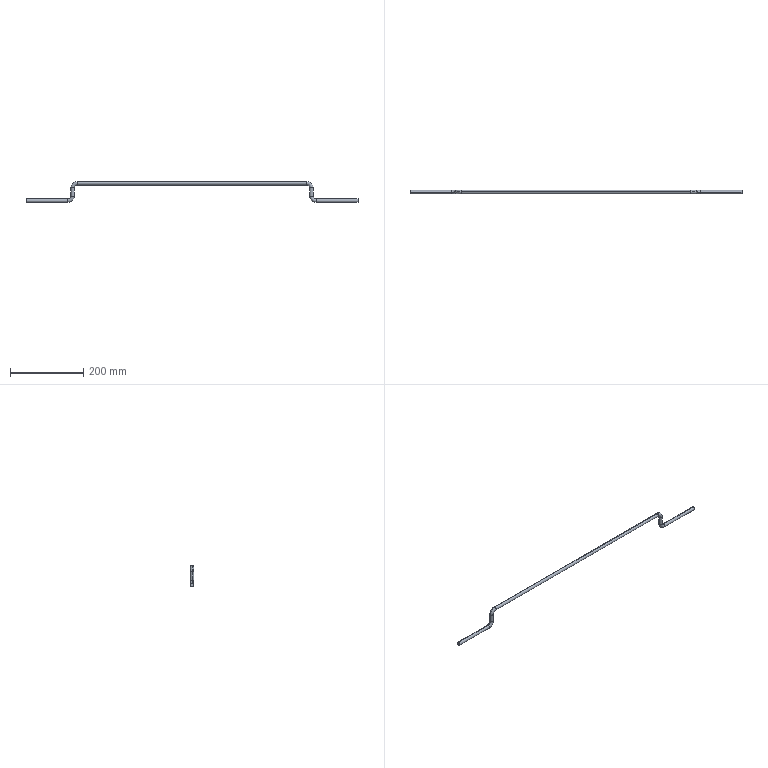Part | NX | features BREP 1 | 1 solid | 20 faces | box 904.875 x 9.525 x 57.15 mm | volume 69711 mm3 | cylinder 10 | torus 8 | plane 2 | commonest cylinder face diameters 9.525 x10
STEP:
#1=CARTESIAN_POINT('',(-452.438,0.,4.763));
#2=VERTEX_POINT('',#1);
#3=CARTESIAN_POINT('',(-452.438,0.,-4.763));
#4=VERTEX_POINT('',#3);
#5=CARTESIAN_POINT('',(-452.438,0.,0.));
#6=DIRECTION('',(1.,0.,0.));
#7=DIRECTION('',(0.,0.,1.));
#8=AXIS2_PLACEMENT_3D('',#5,#6,#7);
#9=CIRCLE('',#8,4.763);
#10=EDGE_CURVE('',#2,#4,#9,.T.);
#11=ORIENTED_EDGE('',*,*,#10,.F.);
#12=CARTESIAN_POINT('',(-452.438,0.,0.));
#13=DIRECTION('',(1.,0.,0.));
#14=DIRECTION('',(0.,0.,-1.));
#15=AXIS2_PLACEMENT_3D('',#12,#13,#14);
#16=CIRCLE('',#15,4.763);
#17=EDGE_CURVE('',#4,#2,#16,.T.);
#18=ORIENTED_EDGE('',*,*,#17,.F.);
#19=EDGE_LOOP('',(#11,#18));
#20=FACE_BOUND('',#19,.T.);
#21=CARTESIAN_POINT('',(-452.438,0.,0.));
#22=DIRECTION('',(1.,0.,0.));
#23=DIRECTION('',(0.,1.,0.));
#24=AXIS2_PLACEMENT_3D('',#21,#22,#23);
#25=PLANE('',#24);
#26=ADVANCED_FACE('',(#20),#25,.F.);
#27=CARTESIAN_POINT('',(-338.137,0.,4.763));
#28=VERTEX_POINT('',#27);
#29=CARTESIAN_POINT('',(-452.438,0.,4.763));
#30=DIRECTION('',(1.,0.,0.));
#31=VECTOR('',#30,1000.);
#32=LINE('',#29,#31);
#33=EDGE_CURVE('',#28,#2,#32,.F.);
#34=ORIENTED_EDGE('',*,*,#33,.F.);
#35=CARTESIAN_POINT('',(-338.137,0.,-4.763));
#36=VERTEX_POINT('',#35);
#37=CARTESIAN_POINT('',(-338.137,0.,0.));
#38=DIRECTION('',(1.,0.,0.));
#39=DIRECTION('',(0.,0.,-1.));
#40=AXIS2_PLACEMENT_3D('',#37,#38,#39);
#41=CIRCLE('',#40,4.763);
#42=EDGE_CURVE('',#36,#28,#41,.T.);
#43=ORIENTED_EDGE('',*,*,#42,.F.);
#44=CARTESIAN_POINT('',(-452.438,0.,-4.763));
#45=DIRECTION('',(1.,0.,0.));
#46=VECTOR('',#45,1000.);
#47=LINE('',#44,#46);
#48=EDGE_CURVE('',#36,#4,#47,.F.);
#49=ORIENTED_EDGE('',*,*,#48,.T.);
#50=ORIENTED_EDGE('',*,*,#17,.T.);
#51=EDGE_LOOP('',(#34,#43,#49,#50));
#52=FACE_BOUND('',#51,.T.);
#53=CARTESIAN_POINT('',(-452.438,0.,0.));
#54=DIRECTION('',(1.,0.,0.));
#55=DIRECTION('',(0.,0.,-1.));
#56=AXIS2_PLACEMENT_3D('',#53,#54,#55);
#57=CYLINDRICAL_SURFACE('',#56,4.763);
#58=ADVANCED_FACE('',(#52),#57,.T.);
#59=ORIENTED_EDGE('',*,*,#48,.F.);
#60=CARTESIAN_POINT('',(-338.137,0.,0.));
#61=DIRECTION('',(1.,0.,0.));
#62=DIRECTION('',(0.,0.,1.));
#63=AXIS2_PLACEMENT_3D('',#60,#61,#62);
#64=CIRCLE('',#63,4.763);
#65=EDGE_CURVE('',#28,#36,#64,.T.);
#66=ORIENTED_EDGE('',*,*,#65,.F.);
#67=ORIENTED_EDGE('',*,*,#33,.T.);
#68=ORIENTED_EDGE('',*,*,#10,.T.);
#69=EDGE_LOOP('',(#59,#66,#67,#68));
#70=FACE_BOUND('',#69,.T.);
#71=CARTESIAN_POINT('',(-452.438,0.,0.));
#72=DIRECTION('',(1.,0.,0.));
#73=DIRECTION('',(0.,0.,-1.));
#74=AXIS2_PLACEMENT_3D('',#71,#72,#73);
#75=CYLINDRICAL_SURFACE('',#74,4.763);
#76=ADVANCED_FACE('',(#70),#75,.T.);
#77=CARTESIAN_POINT('',(-320.675,0.,12.7));
#78=VERTEX_POINT('',#77);
#79=CARTESIAN_POINT('',(-338.137,0.,12.7));
#80=DIRECTION('',(0.,-1.,0.));
#81=DIRECTION('',(0.,0.,-1.));
#82=AXIS2_PLACEMENT_3D('',#79,#80,#81);
#83=CIRCLE('',#82,17.462);
#84=EDGE_CURVE('',#36,#78,#83,.T.);
#85=ORIENTED_EDGE('',*,*,#84,.T.);
#86=CARTESIAN_POINT('',(-330.2,0.,12.7));
#87=VERTEX_POINT('',#86);
#88=CARTESIAN_POINT('',(-325.438,0.,12.7));
#89=DIRECTION('',(0.,0.,1.));
#90=DIRECTION('',(-1.,0.,0.));
#91=AXIS2_PLACEMENT_3D('',#88,#89,#90);
#92=CIRCLE('',#91,4.763);
#93=EDGE_CURVE('',#87,#78,#92,.T.);
#94=ORIENTED_EDGE('',*,*,#93,.F.);
#95=CARTESIAN_POINT('',(-338.137,0.,12.7));
#96=DIRECTION('',(0.,-1.,0.));
#97=DIRECTION('',(0.,0.,-1.));
#98=AXIS2_PLACEMENT_3D('',#95,#96,#97);
#99=CIRCLE('',#98,7.938);
#100=EDGE_CURVE('',#28,#87,#99,.T.);
#101=ORIENTED_EDGE('',*,*,#100,.F.);
#102=ORIENTED_EDGE('',*,*,#65,.T.);
#103=EDGE_LOOP('',(#85,#94,#101,#102));
#104=FACE_BOUND('',#103,.T.);
#105=CARTESIAN_POINT('',(-338.137,0.,12.7));
#106=DIRECTION('',(0.,-1.,0.));
#107=DIRECTION('',(0.,0.,1.));
#108=AXIS2_PLACEMENT_3D('',#105,#106,#107);
#109=TOROIDAL_SURFACE('',#108,12.7,4.763);
#110=ADVANCED_FACE('',(#104),#109,.T.);
#111=ORIENTED_EDGE('',*,*,#100,.T.);
#112=CARTESIAN_POINT('',(-325.438,0.,12.7));
#113=DIRECTION('',(0.,0.,1.));
#114=DIRECTION('',(1.,0.,0.));
#115=AXIS2_PLACEMENT_3D('',#112,#113,#114);
#116=CIRCLE('',#115,4.763);
#117=EDGE_CURVE('',#78,#87,#116,.T.);
#118=ORIENTED_EDGE('',*,*,#117,.F.);
#119=ORIENTED_EDGE('',*,*,#84,.F.);
#120=ORIENTED_EDGE('',*,*,#42,.T.);
#121=EDGE_LOOP('',(#111,#118,#119,#120));
#122=FACE_BOUND('',#121,.T.);
#123=CARTESIAN_POINT('',(-338.137,0.,12.7));
#124=DIRECTION('',(0.,-1.,0.));
#125=DIRECTION('',(0.,0.,1.));
#126=AXIS2_PLACEMENT_3D('',#123,#124,#125);
#127=TOROIDAL_SURFACE('',#126,12.7,4.763);
#128=ADVANCED_FACE('',(#122),#127,.T.);
#129=CARTESIAN_POINT('',(-330.2,0.,34.925));
#130=VERTEX_POINT('',#129);
#131=CARTESIAN_POINT('',(-330.2,0.,12.7));
#132=DIRECTION('',(0.,0.,1.));
#133=VECTOR('',#132,1000.);
#134=LINE('',#131,#133);
#135=EDGE_CURVE('',#87,#130,#134,.T.);
#136=ORIENTED_EDGE('',*,*,#135,.T.);
#137=CARTESIAN_POINT('',(-320.675,0.,34.925));
#138=VERTEX_POINT('',#137);
#139=CARTESIAN_POINT('',(-325.438,0.,34.925));
#140=DIRECTION('',(0.,0.,1.));
#141=DIRECTION('',(1.,0.,0.));
#142=AXIS2_PLACEMENT_3D('',#139,#140,#141);
#143=CIRCLE('',#142,4.763);
#144=EDGE_CURVE('',#138,#130,#143,.T.);
#145=ORIENTED_EDGE('',*,*,#144,.F.);
#146=CARTESIAN_POINT('',(-320.675,0.,12.7));
#147=DIRECTION('',(0.,0.,1.));
#148=VECTOR('',#147,1000.);
#149=LINE('',#146,#148);
#150=EDGE_CURVE('',#78,#138,#149,.T.);
#151=ORIENTED_EDGE('',*,*,#150,.F.);
#152=ORIENTED_EDGE('',*,*,#117,.T.);
#153=EDGE_LOOP('',(#136,#145,#151,#152));
#154=FACE_BOUND('',#153,.T.);
#155=CARTESIAN_POINT('',(-325.438,0.,12.7));
#156=DIRECTION('',(0.,0.,1.));
#157=DIRECTION('',(1.,0.,0.));
#158=AXIS2_PLACEMENT_3D('',#155,#156,#157);
#159=CYLINDRICAL_SURFACE('',#158,4.763);
#160=ADVANCED_FACE('',(#154),#159,.T.);
#161=ORIENTED_EDGE('',*,*,#150,.T.);
#162=CARTESIAN_POINT('',(-325.438,0.,34.925));
#163=DIRECTION('',(0.,0.,1.));
#164=DIRECTION('',(-1.,0.,0.));
#165=AXIS2_PLACEMENT_3D('',#162,#163,#164);
#166=CIRCLE('',#165,4.763);
#167=EDGE_CURVE('',#130,#138,#166,.T.);
#168=ORIENTED_EDGE('',*,*,#167,.F.);
#169=ORIENTED_EDGE('',*,*,#135,.F.);
#170=ORIENTED_EDGE('',*,*,#93,.T.);
#171=EDGE_LOOP('',(#161,#168,#169,#170));
#172=FACE_BOUND('',#171,.T.);
#173=CARTESIAN_POINT('',(-325.438,0.,12.7));
#174=DIRECTION('',(0.,0.,1.));
#175=DIRECTION('',(1.,0.,0.));
#176=AXIS2_PLACEMENT_3D('',#173,#174,#175);
#177=CYLINDRICAL_SURFACE('',#176,4.763);
#178=ADVANCED_FACE('',(#172),#177,.T.);
#179=CARTESIAN_POINT('',(-312.738,0.,42.862));
#180=VERTEX_POINT('',#179);
#181=CARTESIAN_POINT('',(-312.738,0.,34.925));
#182=DIRECTION('',(0.,1.,0.));
#183=DIRECTION('',(-1.,0.,0.));
#184=AXIS2_PLACEMENT_3D('',#181,#182,#183);
#185=CIRCLE('',#184,7.937);
#186=EDGE_CURVE('',#180,#138,#185,.F.);
#187=ORIENTED_EDGE('',*,*,#186,.F.);
#188=CARTESIAN_POINT('',(-312.738,0.,52.388));
#189=VERTEX_POINT('',#188);
#190=CARTESIAN_POINT('',(-312.738,0.,47.625));
#191=DIRECTION('',(1.,0.,0.));
#192=DIRECTION('',(0.,0.,1.));
#193=AXIS2_PLACEMENT_3D('',#190,#191,#192);
#194=CIRCLE('',#193,4.763);
#195=EDGE_CURVE('',#189,#180,#194,.T.);
#196=ORIENTED_EDGE('',*,*,#195,.F.);
#197=CARTESIAN_POINT('',(-312.738,0.,34.925));
#198=DIRECTION('',(0.,1.,0.));
#199=DIRECTION('',(-1.,0.,0.));
#200=AXIS2_PLACEMENT_3D('',#197,#198,#199);
#201=CIRCLE('',#200,17.462);
#202=EDGE_CURVE('',#189,#130,#201,.F.);
#203=ORIENTED_EDGE('',*,*,#202,.T.);
#204=ORIENTED_EDGE('',*,*,#167,.T.);
#205=EDGE_LOOP('',(#187,#196,#203,#204));
#206=FACE_BOUND('',#205,.T.);
#207=CARTESIAN_POINT('',(-312.738,0.,34.925));
#208=DIRECTION('',(0.,1.,0.));
#209=DIRECTION('',(1.,0.,0.));
#210=AXIS2_PLACEMENT_3D('',#207,#208,#209);
#211=TOROIDAL_SURFACE('',#210,12.7,4.763);
#212=ADVANCED_FACE('',(#206),#211,.T.);
#213=ORIENTED_EDGE('',*,*,#202,.F.);
#214=CARTESIAN_POINT('',(-312.738,0.,47.625));
#215=DIRECTION('',(1.,0.,0.));
#216=DIRECTION('',(0.,0.,-1.));
#217=AXIS2_PLACEMENT_3D('',#214,#215,#216);
#218=CIRCLE('',#217,4.763);
#219=EDGE_CURVE('',#180,#189,#218,.T.);
#220=ORIENTED_EDGE('',*,*,#219,.F.);
#221=ORIENTED_EDGE('',*,*,#186,.T.);
#222=ORIENTED_EDGE('',*,*,#144,.T.);
#223=EDGE_LOOP('',(#213,#220,#221,#222));
#224=FACE_BOUND('',#223,.T.);
#225=CARTESIAN_POINT('',(-312.738,0.,34.925));
#226=DIRECTION('',(0.,1.,0.));
#227=DIRECTION('',(1.,0.,0.));
#228=AXIS2_PLACEMENT_3D('',#225,#226,#227);
#229=TOROIDAL_SURFACE('',#228,12.7,4.763);
#230=ADVANCED_FACE('',(#224),#229,.T.);
#231=CARTESIAN_POINT('',(312.738,0.,52.388));
#232=VERTEX_POINT('',#231);
#233=CARTESIAN_POINT('',(-312.738,0.,52.388));
#234=DIRECTION('',(1.,0.,0.));
#235=VECTOR('',#234,1000.);
#236=LINE('',#233,#235);
#237=EDGE_CURVE('',#232,#189,#236,.F.);
#238=ORIENTED_EDGE('',*,*,#237,.F.);
#239=CARTESIAN_POINT('',(312.738,0.,42.862));
#240=VERTEX_POINT('',#239);
#241=CARTESIAN_POINT('',(312.738,0.,47.625));
#242=DIRECTION('',(1.,0.,0.));
#243=DIRECTION('',(0.,0.,-1.));
#244=AXIS2_PLACEMENT_3D('',#241,#242,#243);
#245=CIRCLE('',#244,4.763);
#246=EDGE_CURVE('',#240,#232,#245,.T.);
#247=ORIENTED_EDGE('',*,*,#246,.F.);
#248=CARTESIAN_POINT('',(-312.738,0.,42.862));
#249=DIRECTION('',(1.,0.,0.));
#250=VECTOR('',#249,1000.);
#251=LINE('',#248,#250);
#252=EDGE_CURVE('',#240,#180,#251,.F.);
#253=ORIENTED_EDGE('',*,*,#252,.T.);
#254=ORIENTED_EDGE('',*,*,#219,.T.);
#255=EDGE_LOOP('',(#238,#247,#253,#254));
#256=FACE_BOUND('',#255,.T.);
#257=CARTESIAN_POINT('',(-312.738,0.,47.625));
#258=DIRECTION('',(1.,0.,0.));
#259=DIRECTION('',(0.,0.,-1.));
#260=AXIS2_PLACEMENT_3D('',#257,#258,#259);
#261=CYLINDRICAL_SURFACE('',#260,4.763);
#262=ADVANCED_FACE('',(#256),#261,.T.);
#263=ORIENTED_EDGE('',*,*,#252,.F.);
#264=CARTESIAN_POINT('',(312.738,0.,47.625));
#265=DIRECTION('',(1.,0.,0.));
#266=DIRECTION('',(0.,0.,1.));
#267=AXIS2_PLACEMENT_3D('',#264,#265,#266);
#268=CIRCLE('',#267,4.763);
#269=EDGE_CURVE('',#232,#240,#268,.T.);
#270=ORIENTED_EDGE('',*,*,#269,.F.);
#271=ORIENTED_EDGE('',*,*,#237,.T.);
#272=ORIENTED_EDGE('',*,*,#195,.T.);
#273=EDGE_LOOP('',(#263,#270,#271,#272));
#274=FACE_BOUND('',#273,.T.);
#275=CARTESIAN_POINT('',(-312.738,0.,47.625));
#276=DIRECTION('',(1.,0.,0.));
#277=DIRECTION('',(0.,0.,-1.));
#278=AXIS2_PLACEMENT_3D('',#275,#276,#277);
#279=CYLINDRICAL_SURFACE('',#278,4.763);
#280=ADVANCED_FACE('',(#274),#279,.T.);
#281=CARTESIAN_POINT('',(320.675,0.,34.925));
#282=VERTEX_POINT('',#281);
#283=CARTESIAN_POINT('',(312.738,0.,34.925));
#284=DIRECTION('',(0.,1.,0.));
#285=DIRECTION('',(0.,0.,1.));
#286=AXIS2_PLACEMENT_3D('',#283,#284,#285);
#287=CIRCLE('',#286,7.938);
#288=EDGE_CURVE('',#240,#282,#287,.T.);
#289=ORIENTED_EDGE('',*,*,#288,.T.);
#290=CARTESIAN_POINT('',(330.2,0.,34.925));
#291=VERTEX_POINT('',#290);
#292=CARTESIAN_POINT('',(325.438,0.,34.925));
#293=DIRECTION('',(0.,0.,-1.));
#294=DIRECTION('',(1.,0.,0.));
#295=AXIS2_PLACEMENT_3D('',#292,#293,#294);
#296=CIRCLE('',#295,4.763);
#297=EDGE_CURVE('',#291,#282,#296,.T.);
#298=ORIENTED_EDGE('',*,*,#297,.F.);
#299=CARTESIAN_POINT('',(312.738,0.,34.925));
#300=DIRECTION('',(0.,1.,0.));
#301=DIRECTION('',(0.,0.,1.));
#302=AXIS2_PLACEMENT_3D('',#299,#300,#301);
#303=CIRCLE('',#302,17.462);
#304=EDGE_CURVE('',#232,#291,#303,.T.);
#305=ORIENTED_EDGE('',*,*,#304,.F.);
#306=ORIENTED_EDGE('',*,*,#269,.T.);
#307=EDGE_LOOP('',(#289,#298,#305,#306));
#308=FACE_BOUND('',#307,.T.);
#309=CARTESIAN_POINT('',(312.738,0.,34.925));
#310=DIRECTION('',(0.,1.,0.));
#311=DIRECTION('',(0.,0.,-1.));
#312=AXIS2_PLACEMENT_3D('',#309,#310,#311);
#313=TOROIDAL_SURFACE('',#312,12.7,4.763);
#314=ADVANCED_FACE('',(#308),#313,.T.);
#315=ORIENTED_EDGE('',*,*,#304,.T.);
#316=CARTESIAN_POINT('',(325.438,0.,34.925));
#317=DIRECTION('',(0.,0.,-1.));
#318=DIRECTION('',(-1.,0.,0.));
#319=AXIS2_PLACEMENT_3D('',#316,#317,#318);
#320=CIRCLE('',#319,4.763);
#321=EDGE_CURVE('',#282,#291,#320,.T.);
#322=ORIENTED_EDGE('',*,*,#321,.F.);
#323=ORIENTED_EDGE('',*,*,#288,.F.);
#324=ORIENTED_EDGE('',*,*,#246,.T.);
#325=EDGE_LOOP('',(#315,#322,#323,#324));
#326=FACE_BOUND('',#325,.T.);
#327=CARTESIAN_POINT('',(312.738,0.,34.925));
#328=DIRECTION('',(0.,1.,0.));
#329=DIRECTION('',(0.,0.,-1.));
#330=AXIS2_PLACEMENT_3D('',#327,#328,#329);
#331=TOROIDAL_SURFACE('',#330,12.7,4.763);
#332=ADVANCED_FACE('',(#326),#331,.T.);
#333=CARTESIAN_POINT('',(330.2,0.,12.7));
#334=VERTEX_POINT('',#333);
#335=CARTESIAN_POINT('',(330.2,0.,34.925));
#336=DIRECTION('',(0.,0.,-1.));
#337=VECTOR('',#336,1000.);
#338=LINE('',#335,#337);
#339=EDGE_CURVE('',#334,#291,#338,.F.);
#340=ORIENTED_EDGE('',*,*,#339,.F.);
#341=CARTESIAN_POINT('',(320.675,0.,12.7));
#342=VERTEX_POINT('',#341);
#343=CARTESIAN_POINT('',(325.438,0.,12.7));
#344=DIRECTION('',(0.,0.,-1.));
#345=DIRECTION('',(-1.,0.,0.));
#346=AXIS2_PLACEMENT_3D('',#343,#344,#345);
#347=CIRCLE('',#346,4.763);
#348=EDGE_CURVE('',#342,#334,#347,.T.);
#349=ORIENTED_EDGE('',*,*,#348,.F.);
#350=CARTESIAN_POINT('',(320.675,0.,34.925));
#351=DIRECTION('',(0.,0.,-1.));
#352=VECTOR('',#351,1000.);
#353=LINE('',#350,#352);
#354=EDGE_CURVE('',#342,#282,#353,.F.);
#355=ORIENTED_EDGE('',*,*,#354,.T.);
#356=ORIENTED_EDGE('',*,*,#321,.T.);
#357=EDGE_LOOP('',(#340,#349,#355,#356));
#358=FACE_BOUND('',#357,.T.);
#359=CARTESIAN_POINT('',(325.438,0.,34.925));
#360=DIRECTION('',(0.,0.,-1.));
#361=DIRECTION('',(-1.,0.,0.));
#362=AXIS2_PLACEMENT_3D('',#359,#360,#361);
#363=CYLINDRICAL_SURFACE('',#362,4.763);
#364=ADVANCED_FACE('',(#358),#363,.T.);
#365=ORIENTED_EDGE('',*,*,#354,.F.);
#366=CARTESIAN_POINT('',(325.438,0.,12.7));
#367=DIRECTION('',(0.,0.,-1.));
#368=DIRECTION('',(1.,0.,0.));
#369=AXIS2_PLACEMENT_3D('',#366,#367,#368);
#370=CIRCLE('',#369,4.763);
#371=EDGE_CURVE('',#334,#342,#370,.T.);
#372=ORIENTED_EDGE('',*,*,#371,.F.);
#373=ORIENTED_EDGE('',*,*,#339,.T.);
#374=ORIENTED_EDGE('',*,*,#297,.T.);
#375=EDGE_LOOP('',(#365,#372,#373,#374));
#376=FACE_BOUND('',#375,.T.);
#377=CARTESIAN_POINT('',(325.438,0.,34.925));
#378=DIRECTION('',(0.,0.,-1.));
#379=DIRECTION('',(-1.,0.,0.));
#380=AXIS2_PLACEMENT_3D('',#377,#378,#379);
#381=CYLINDRICAL_SURFACE('',#380,4.763);
#382=ADVANCED_FACE('',(#376),#381,.T.);
#383=CARTESIAN_POINT('',(338.137,0.,-4.763));
#384=VERTEX_POINT('',#383);
#385=CARTESIAN_POINT('',(338.137,0.,12.7));
#386=DIRECTION('',(0.,-1.,0.));
#387=DIRECTION('',(-1.,0.,0.));
#388=AXIS2_PLACEMENT_3D('',#385,#386,#387);
#389=CIRCLE('',#388,17.462);
#390=EDGE_CURVE('',#342,#384,#389,.T.);
#391=ORIENTED_EDGE('',*,*,#390,.T.);
#392=CARTESIAN_POINT('',(338.137,0.,4.763));
#393=VERTEX_POINT('',#392);
#394=CARTESIAN_POINT('',(338.137,0.,0.));
#395=DIRECTION('',(1.,0.,0.));
#396=DIRECTION('',(0.,0.,1.));
#397=AXIS2_PLACEMENT_3D('',#394,#395,#396);
#398=CIRCLE('',#397,4.763);
#399=EDGE_CURVE('',#393,#384,#398,.T.);
#400=ORIENTED_EDGE('',*,*,#399,.F.);
#401=CARTESIAN_POINT('',(338.137,0.,12.7));
#402=DIRECTION('',(0.,-1.,0.));
#403=DIRECTION('',(-1.,0.,0.));
#404=AXIS2_PLACEMENT_3D('',#401,#402,#403);
#405=CIRCLE('',#404,7.937);
#406=EDGE_CURVE('',#334,#393,#405,.T.);
#407=ORIENTED_EDGE('',*,*,#406,.F.);
#408=ORIENTED_EDGE('',*,*,#371,.T.);
#409=EDGE_LOOP('',(#391,#400,#407,#408));
#410=FACE_BOUND('',#409,.T.);
#411=CARTESIAN_POINT('',(338.137,0.,12.7));
#412=DIRECTION('',(0.,-1.,0.));
#413=DIRECTION('',(1.,0.,0.));
#414=AXIS2_PLACEMENT_3D('',#411,#412,#413);
#415=TOROIDAL_SURFACE('',#414,12.7,4.763);
#416=ADVANCED_FACE('',(#410),#415,.T.);
#417=ORIENTED_EDGE('',*,*,#406,.T.);
#418=CARTESIAN_POINT('',(338.137,0.,0.));
#419=DIRECTION('',(1.,0.,0.));
#420=DIRECTION('',(0.,0.,-1.));
#421=AXIS2_PLACEMENT_3D('',#418,#419,#420);
#422=CIRCLE('',#421,4.763);
#423=EDGE_CURVE('',#384,#393,#422,.T.);
#424=ORIENTED_EDGE('',*,*,#423,.F.);
#425=ORIENTED_EDGE('',*,*,#390,.F.);
#426=ORIENTED_EDGE('',*,*,#348,.T.);
#427=EDGE_LOOP('',(#417,#424,#425,#426));
#428=FACE_BOUND('',#427,.T.);
#429=CARTESIAN_POINT('',(338.137,0.,12.7));
#430=DIRECTION('',(0.,-1.,0.));
#431=DIRECTION('',(1.,0.,0.));
#432=AXIS2_PLACEMENT_3D('',#429,#430,#431);
#433=TOROIDAL_SURFACE('',#432,12.7,4.763);
#434=ADVANCED_FACE('',(#428),#433,.T.);
#435=CARTESIAN_POINT('',(452.438,0.,4.763));
#436=VERTEX_POINT('',#435);
#437=CARTESIAN_POINT('',(338.137,0.,4.763));
#438=DIRECTION('',(1.,0.,0.));
#439=VECTOR('',#438,1000.);
#440=LINE('',#437,#439);
#441=EDGE_CURVE('',#436,#393,#440,.F.);
#442=ORIENTED_EDGE('',*,*,#441,.F.);
#443=CARTESIAN_POINT('',(452.438,0.,-4.763));
#444=VERTEX_POINT('',#443);
#445=CARTESIAN_POINT('',(452.438,0.,0.));
#446=DIRECTION('',(1.,0.,0.));
#447=DIRECTION('',(0.,0.,-1.));
#448=AXIS2_PLACEMENT_3D('',#445,#446,#447);
#449=CIRCLE('',#448,4.763);
#450=EDGE_CURVE('',#444,#436,#449,.T.);
#451=ORIENTED_EDGE('',*,*,#450,.F.);
#452=CARTESIAN_POINT('',(338.137,0.,-4.763));
#453=DIRECTION('',(1.,0.,0.));
#454=VECTOR('',#453,1000.);
#455=LINE('',#452,#454);
#456=EDGE_CURVE('',#444,#384,#455,.F.);
#457=ORIENTED_EDGE('',*,*,#456,.T.);
#458=ORIENTED_EDGE('',*,*,#423,.T.);
#459=EDGE_LOOP('',(#442,#451,#457,#458));
#460=FACE_BOUND('',#459,.T.);
#461=CARTESIAN_POINT('',(338.137,0.,0.));
#462=DIRECTION('',(1.,0.,0.));
#463=DIRECTION('',(0.,0.,-1.));
#464=AXIS2_PLACEMENT_3D('',#461,#462,#463);
#465=CYLINDRICAL_SURFACE('',#464,4.763);
#466=ADVANCED_FACE('',(#460),#465,.T.);
#467=ORIENTED_EDGE('',*,*,#456,.F.);
#468=CARTESIAN_POINT('',(452.438,0.,0.));
#469=DIRECTION('',(1.,0.,0.));
#470=DIRECTION('',(0.,0.,1.));
#471=AXIS2_PLACEMENT_3D('',#468,#469,#470);
#472=CIRCLE('',#471,4.763);
#473=EDGE_CURVE('',#436,#444,#472,.T.);
#474=ORIENTED_EDGE('',*,*,#473,.F.);
#475=ORIENTED_EDGE('',*,*,#441,.T.);
#476=ORIENTED_EDGE('',*,*,#399,.T.);
#477=EDGE_LOOP('',(#467,#474,#475,#476));
#478=FACE_BOUND('',#477,.T.);
#479=CARTESIAN_POINT('',(338.137,0.,0.));
#480=DIRECTION('',(1.,0.,0.));
#481=DIRECTION('',(0.,0.,-1.));
#482=AXIS2_PLACEMENT_3D('',#479,#480,#481);
#483=CYLINDRICAL_SURFACE('',#482,4.763);
#484=ADVANCED_FACE('',(#478),#483,.T.);
#485=ORIENTED_EDGE('',*,*,#473,.T.);
#486=ORIENTED_EDGE('',*,*,#450,.T.);
#487=EDGE_LOOP('',(#485,#486));
#488=FACE_BOUND('',#487,.T.);
#489=CARTESIAN_POINT('',(452.438,0.,0.));
#490=DIRECTION('',(1.,0.,0.));
#491=DIRECTION('',(0.,1.,0.));
#492=AXIS2_PLACEMENT_3D('',#489,#490,#491);
#493=PLANE('',#492);
#494=ADVANCED_FACE('',(#488),#493,.T.);
#495=CLOSED_SHELL('',(#26,#58,#76,#110,#128,#160,#178,#212,#230,#262,#280,#314,#332,#364,#382,#416,#434,#466,#484,#494));
#496=MANIFOLD_SOLID_BREP('',#495);
#497=(LENGTH_UNIT()NAMED_UNIT(*)SI_UNIT(.MILLI.,.METRE.));
#498=UNCERTAINTY_MEASURE_WITH_UNIT(LENGTH_MEASURE(0.00001),#497,'','');
#499=(NAMED_UNIT(*)PLANE_ANGLE_UNIT()SI_UNIT($,.RADIAN.));
#500=(NAMED_UNIT(*)SI_UNIT($,.STERADIAN.)SOLID_ANGLE_UNIT());
#501=(GEOMETRIC_REPRESENTATION_CONTEXT(3)GLOBAL_UNCERTAINTY_ASSIGNED_CONTEXT((#498))GLOBAL_UNIT_ASSIGNED_CONTEXT((#497,#499,#500))REPRESENTATION_CONTEXT('',''));
#502=ADVANCED_BREP_SHAPE_REPRESENTATION('',(#496),#501);